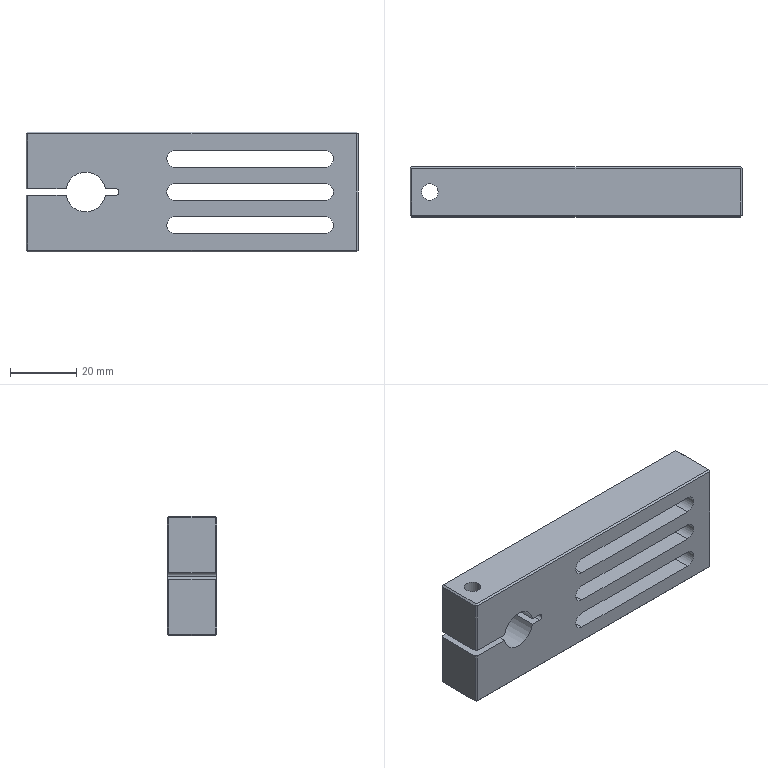Part | STEP file | ND25021-01-JDKM-51-TL | 1 solid | 53 faces | box 100 x 15 x 36 mm | volume 38964 mm3 | plane 36 | cylinder 17 | commonest cylinder face diameters 5.2 x6 12 x3 2 x2 5 x2 6.6 x2 11 x2